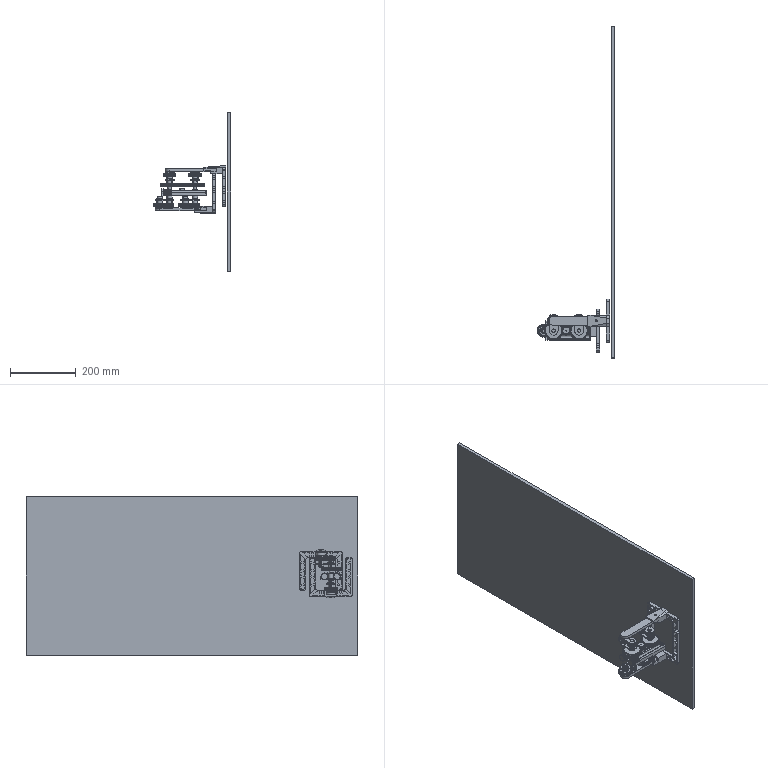Part | NX | features DATUM_CSYS 24, EXTRUDE 13, SKETCH 11, BREP 10, REPLACE_FACE 5, UNITE 3, CHAMFER 1, CYLINDER 1, DATUM_PLANE 1, OFFSET 1, SUBTRACT 1, THREADS 1 | 37 solids | 2334 faces | box 235.972 x 1013 x 485 mm | volume 5370772 mm3 | cylinder 1831 | plane 495 | spline 6 | cone 2 | commonest cylinder face diameters 4 x360 14.148 x192 6 x144 18.651 x144 11.066 x128 1.7 x96